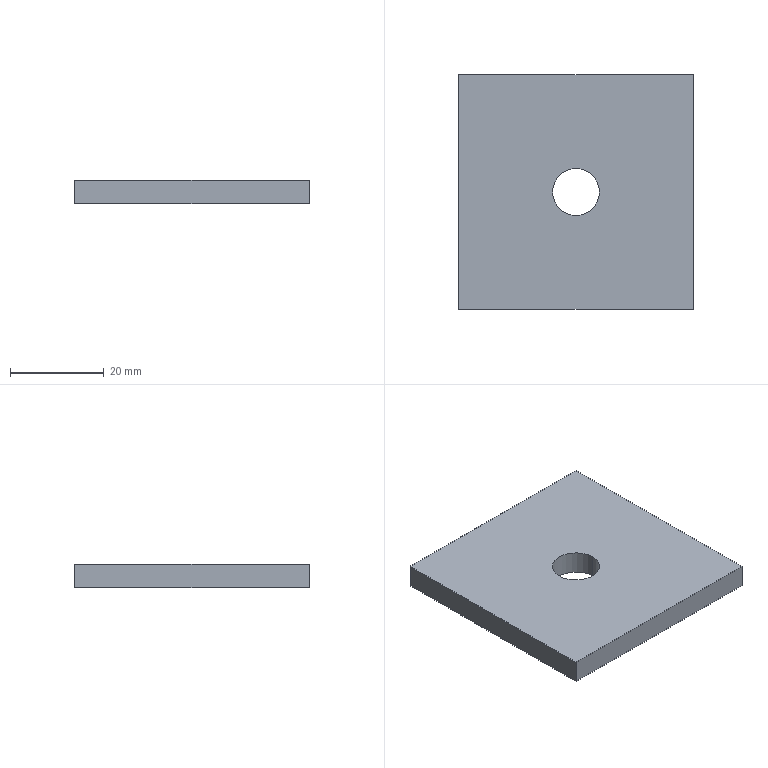Part | NX | features BREP 1 | 1 solid | 8 faces | box 50 x 50 x 5 mm | volume 12107 mm3 | plane 6 | cylinder 2 | commonest cylinder face diameters 10 x2
STEP:
#1=CARTESIAN_POINT('',(-5.,0.,0.));
#2=VERTEX_POINT('',#1);
#3=CARTESIAN_POINT('',(-5.,0.,5.));
#4=VERTEX_POINT('',#3);
#5=CARTESIAN_POINT('',(-5.,0.,0.));
#6=DIRECTION('',(0.,0.,1.));
#7=VECTOR('',#6,1000.);
#8=LINE('',#5,#7);
#9=EDGE_CURVE('',#2,#4,#8,.T.);
#10=ORIENTED_EDGE('',*,*,#9,.T.);
#11=CARTESIAN_POINT('',(5.,0.,5.));
#12=VERTEX_POINT('',#11);
#13=CARTESIAN_POINT('',(0.,0.,5.));
#14=DIRECTION('',(0.,0.,-1.));
#15=DIRECTION('',(1.,0.,0.));
#16=AXIS2_PLACEMENT_3D('',#13,#14,#15);
#17=CIRCLE('',#16,5.);
#18=EDGE_CURVE('',#12,#4,#17,.T.);
#19=ORIENTED_EDGE('',*,*,#18,.F.);
#20=CARTESIAN_POINT('',(5.,0.,0.));
#21=VERTEX_POINT('',#20);
#22=CARTESIAN_POINT('',(5.,0.,0.));
#23=DIRECTION('',(0.,0.,1.));
#24=VECTOR('',#23,1000.);
#25=LINE('',#22,#24);
#26=EDGE_CURVE('',#21,#12,#25,.T.);
#27=ORIENTED_EDGE('',*,*,#26,.F.);
#28=CARTESIAN_POINT('',(0.,0.,0.));
#29=DIRECTION('',(0.,0.,1.));
#30=DIRECTION('',(-1.,0.,0.));
#31=AXIS2_PLACEMENT_3D('',#28,#29,#30);
#32=CIRCLE('',#31,5.);
#33=EDGE_CURVE('',#2,#21,#32,.T.);
#34=ORIENTED_EDGE('',*,*,#33,.F.);
#35=EDGE_LOOP('',(#10,#19,#27,#34));
#36=FACE_BOUND('',#35,.T.);
#37=CARTESIAN_POINT('',(0.,0.,1.84));
#38=DIRECTION('',(0.,0.,1.));
#39=DIRECTION('',(1.,0.,0.));
#40=AXIS2_PLACEMENT_3D('',#37,#38,#39);
#41=CYLINDRICAL_SURFACE('',#40,5.);
#42=ADVANCED_FACE('',(#36),#41,.F.);
#43=CARTESIAN_POINT('',(25.,-25.,0.));
#44=VERTEX_POINT('',#43);
#45=CARTESIAN_POINT('',(-25.,-25.,0.));
#46=VERTEX_POINT('',#45);
#47=CARTESIAN_POINT('',(25.,-25.,0.));
#48=DIRECTION('',(-1.,0.,0.));
#49=VECTOR('',#48,1000.);
#50=LINE('',#47,#49);
#51=EDGE_CURVE('',#44,#46,#50,.T.);
#52=ORIENTED_EDGE('',*,*,#51,.T.);
#53=CARTESIAN_POINT('',(-25.,25.,0.));
#54=VERTEX_POINT('',#53);
#55=CARTESIAN_POINT('',(-25.,-25.,0.));
#56=DIRECTION('',(0.,1.,0.));
#57=VECTOR('',#56,1000.);
#58=LINE('',#55,#57);
#59=EDGE_CURVE('',#46,#54,#58,.T.);
#60=ORIENTED_EDGE('',*,*,#59,.T.);
#61=CARTESIAN_POINT('',(25.,25.,0.));
#62=VERTEX_POINT('',#61);
#63=CARTESIAN_POINT('',(-25.,25.,0.));
#64=DIRECTION('',(1.,0.,0.));
#65=VECTOR('',#64,1000.);
#66=LINE('',#63,#65);
#67=EDGE_CURVE('',#54,#62,#66,.T.);
#68=ORIENTED_EDGE('',*,*,#67,.T.);
#69=CARTESIAN_POINT('',(25.,25.,0.));
#70=DIRECTION('',(0.,-1.,0.));
#71=VECTOR('',#70,1000.);
#72=LINE('',#69,#71);
#73=EDGE_CURVE('',#62,#44,#72,.T.);
#74=ORIENTED_EDGE('',*,*,#73,.T.);
#75=EDGE_LOOP('',(#52,#60,#68,#74));
#76=FACE_BOUND('',#75,.T.);
#77=CARTESIAN_POINT('',(0.,0.,0.));
#78=DIRECTION('',(0.,0.,1.));
#79=DIRECTION('',(1.,0.,0.));
#80=AXIS2_PLACEMENT_3D('',#77,#78,#79);
#81=CIRCLE('',#80,5.);
#82=EDGE_CURVE('',#21,#2,#81,.T.);
#83=ORIENTED_EDGE('',*,*,#82,.T.);
#84=ORIENTED_EDGE('',*,*,#33,.T.);
#85=EDGE_LOOP('',(#83,#84));
#86=FACE_BOUND('',#85,.T.);
#87=CARTESIAN_POINT('',(0.,0.,0.));
#88=DIRECTION('',(0.,0.,1.));
#89=DIRECTION('',(1.,0.,0.));
#90=AXIS2_PLACEMENT_3D('',#87,#88,#89);
#91=PLANE('',#90);
#92=ADVANCED_FACE('',(#76,#86),#91,.F.);
#93=ORIENTED_EDGE('',*,*,#73,.F.);
#94=CARTESIAN_POINT('',(25.,25.,5.));
#95=VERTEX_POINT('',#94);
#96=CARTESIAN_POINT('',(25.,25.,5.));
#97=DIRECTION('',(0.,0.,-1.));
#98=VECTOR('',#97,1000.);
#99=LINE('',#96,#98);
#100=EDGE_CURVE('',#95,#62,#99,.T.);
#101=ORIENTED_EDGE('',*,*,#100,.F.);
#102=CARTESIAN_POINT('',(25.,-25.,5.));
#103=VERTEX_POINT('',#102);
#104=CARTESIAN_POINT('',(25.,25.,5.));
#105=DIRECTION('',(0.,-1.,0.));
#106=VECTOR('',#105,1000.);
#107=LINE('',#104,#106);
#108=EDGE_CURVE('',#95,#103,#107,.T.);
#109=ORIENTED_EDGE('',*,*,#108,.T.);
#110=CARTESIAN_POINT('',(25.,-25.,5.));
#111=DIRECTION('',(0.,0.,-1.));
#112=VECTOR('',#111,1000.);
#113=LINE('',#110,#112);
#114=EDGE_CURVE('',#103,#44,#113,.T.);
#115=ORIENTED_EDGE('',*,*,#114,.T.);
#116=EDGE_LOOP('',(#93,#101,#109,#115));
#117=FACE_BOUND('',#116,.T.);
#118=CARTESIAN_POINT('',(25.,25.,0.));
#119=DIRECTION('',(-1.,0.,0.));
#120=DIRECTION('',(0.,0.,1.));
#121=AXIS2_PLACEMENT_3D('',#118,#119,#120);
#122=PLANE('',#121);
#123=ADVANCED_FACE('',(#117),#122,.F.);
#124=ORIENTED_EDGE('',*,*,#51,.F.);
#125=ORIENTED_EDGE('',*,*,#114,.F.);
#126=CARTESIAN_POINT('',(-25.,-25.,5.));
#127=VERTEX_POINT('',#126);
#128=CARTESIAN_POINT('',(25.,-25.,5.));
#129=DIRECTION('',(-1.,0.,0.));
#130=VECTOR('',#129,1000.);
#131=LINE('',#128,#130);
#132=EDGE_CURVE('',#103,#127,#131,.T.);
#133=ORIENTED_EDGE('',*,*,#132,.T.);
#134=CARTESIAN_POINT('',(-25.,-25.,5.));
#135=DIRECTION('',(0.,0.,-1.));
#136=VECTOR('',#135,1000.);
#137=LINE('',#134,#136);
#138=EDGE_CURVE('',#127,#46,#137,.T.);
#139=ORIENTED_EDGE('',*,*,#138,.T.);
#140=EDGE_LOOP('',(#124,#125,#133,#139));
#141=FACE_BOUND('',#140,.T.);
#142=CARTESIAN_POINT('',(25.,-25.,0.));
#143=DIRECTION('',(0.,1.,0.));
#144=DIRECTION('',(1.,0.,0.));
#145=AXIS2_PLACEMENT_3D('',#142,#143,#144);
#146=PLANE('',#145);
#147=ADVANCED_FACE('',(#141),#146,.F.);
#148=ORIENTED_EDGE('',*,*,#59,.F.);
#149=ORIENTED_EDGE('',*,*,#138,.F.);
#150=CARTESIAN_POINT('',(-25.,25.,5.));
#151=VERTEX_POINT('',#150);
#152=CARTESIAN_POINT('',(-25.,-25.,5.));
#153=DIRECTION('',(0.,1.,0.));
#154=VECTOR('',#153,1000.);
#155=LINE('',#152,#154);
#156=EDGE_CURVE('',#127,#151,#155,.T.);
#157=ORIENTED_EDGE('',*,*,#156,.T.);
#158=CARTESIAN_POINT('',(-25.,25.,5.));
#159=DIRECTION('',(0.,0.,-1.));
#160=VECTOR('',#159,1000.);
#161=LINE('',#158,#160);
#162=EDGE_CURVE('',#151,#54,#161,.T.);
#163=ORIENTED_EDGE('',*,*,#162,.T.);
#164=EDGE_LOOP('',(#148,#149,#157,#163));
#165=FACE_BOUND('',#164,.T.);
#166=CARTESIAN_POINT('',(-25.,-25.,0.));
#167=DIRECTION('',(1.,0.,0.));
#168=DIRECTION('',(0.,1.,0.));
#169=AXIS2_PLACEMENT_3D('',#166,#167,#168);
#170=PLANE('',#169);
#171=ADVANCED_FACE('',(#165),#170,.F.);
#172=ORIENTED_EDGE('',*,*,#67,.F.);
#173=ORIENTED_EDGE('',*,*,#162,.F.);
#174=CARTESIAN_POINT('',(-25.,25.,5.));
#175=DIRECTION('',(1.,0.,0.));
#176=VECTOR('',#175,1000.);
#177=LINE('',#174,#176);
#178=EDGE_CURVE('',#151,#95,#177,.T.);
#179=ORIENTED_EDGE('',*,*,#178,.T.);
#180=ORIENTED_EDGE('',*,*,#100,.T.);
#181=EDGE_LOOP('',(#172,#173,#179,#180));
#182=FACE_BOUND('',#181,.T.);
#183=CARTESIAN_POINT('',(-25.,25.,0.));
#184=DIRECTION('',(0.,-1.,0.));
#185=DIRECTION('',(0.,0.,-1.));
#186=AXIS2_PLACEMENT_3D('',#183,#184,#185);
#187=PLANE('',#186);
#188=ADVANCED_FACE('',(#182),#187,.F.);
#189=ORIENTED_EDGE('',*,*,#156,.F.);
#190=ORIENTED_EDGE('',*,*,#132,.F.);
#191=ORIENTED_EDGE('',*,*,#108,.F.);
#192=ORIENTED_EDGE('',*,*,#178,.F.);
#193=EDGE_LOOP('',(#189,#190,#191,#192));
#194=FACE_BOUND('',#193,.T.);
#195=ORIENTED_EDGE('',*,*,#18,.T.);
#196=CARTESIAN_POINT('',(0.,0.,5.));
#197=DIRECTION('',(0.,0.,-1.));
#198=DIRECTION('',(-1.,0.,0.));
#199=AXIS2_PLACEMENT_3D('',#196,#197,#198);
#200=CIRCLE('',#199,5.);
#201=EDGE_CURVE('',#4,#12,#200,.T.);
#202=ORIENTED_EDGE('',*,*,#201,.T.);
#203=EDGE_LOOP('',(#195,#202));
#204=FACE_BOUND('',#203,.T.);
#205=CARTESIAN_POINT('',(0.,0.,5.));
#206=DIRECTION('',(0.,0.,1.));
#207=DIRECTION('',(1.,0.,0.));
#208=AXIS2_PLACEMENT_3D('',#205,#206,#207);
#209=PLANE('',#208);
#210=ADVANCED_FACE('',(#194,#204),#209,.T.);
#211=ORIENTED_EDGE('',*,*,#26,.T.);
#212=ORIENTED_EDGE('',*,*,#201,.F.);
#213=ORIENTED_EDGE('',*,*,#9,.F.);
#214=ORIENTED_EDGE('',*,*,#82,.F.);
#215=EDGE_LOOP('',(#211,#212,#213,#214));
#216=FACE_BOUND('',#215,.T.);
#217=CARTESIAN_POINT('',(0.,0.,1.84));
#218=DIRECTION('',(0.,0.,1.));
#219=DIRECTION('',(1.,0.,0.));
#220=AXIS2_PLACEMENT_3D('',#217,#218,#219);
#221=CYLINDRICAL_SURFACE('',#220,5.);
#222=ADVANCED_FACE('',(#216),#221,.F.);
#223=CLOSED_SHELL('',(#42,#92,#123,#147,#171,#188,#210,#222));
#224=MANIFOLD_SOLID_BREP('',#223);
#225=(LENGTH_UNIT()NAMED_UNIT(*)SI_UNIT(.MILLI.,.METRE.));
#226=UNCERTAINTY_MEASURE_WITH_UNIT(LENGTH_MEASURE(0.00001),#225,'','');
#227=(NAMED_UNIT(*)PLANE_ANGLE_UNIT()SI_UNIT($,.RADIAN.));
#228=(NAMED_UNIT(*)SI_UNIT($,.STERADIAN.)SOLID_ANGLE_UNIT());
#229=(GEOMETRIC_REPRESENTATION_CONTEXT(3)GLOBAL_UNCERTAINTY_ASSIGNED_CONTEXT((#226))GLOBAL_UNIT_ASSIGNED_CONTEXT((#225,#227,#228))REPRESENTATION_CONTEXT('',''));
#230=ADVANCED_BREP_SHAPE_REPRESENTATION('',(#224),#229);